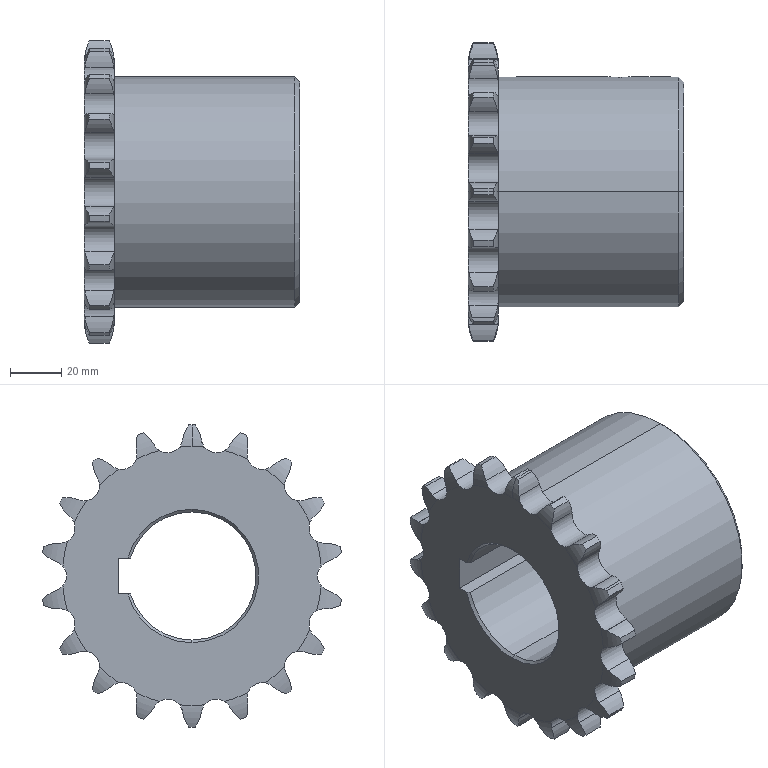Part | SolidWorks | features ICE 2, Chamfer 1, CirPattern 1, HoleWzd 1, RefAxis 1, Revolution 1 | 1 solid | 144 faces | box 84 x 116.558 x 117.94 mm | volume 390436 mm3 | cylinder 92 | torus 38 | cone 8 | plane 6 | commonest cylinder face diameters 28 x40 11.91 x26 117.94 x19 50 x3 10.2 x2 90 x2